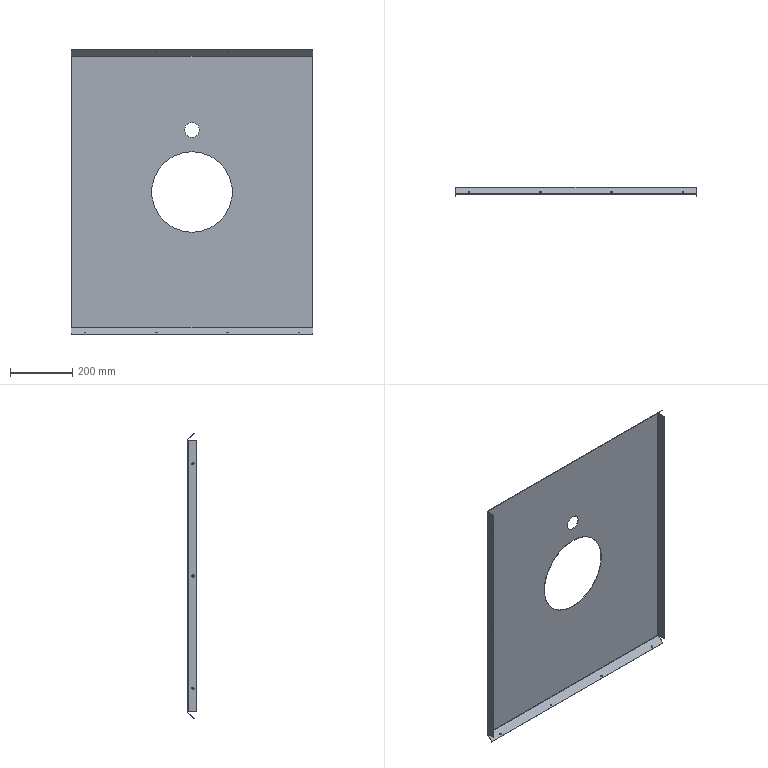Part | SolidWorks | features HoleWzd 3, EdgeFlange 2, Cut 1, FlatPattern 1, ICE 1, SMBaseFlange 1, SheetMetal 1 | 1 solid | 74 faces | box 780 x 30 x 921.426 mm | volume 870668 mm3 | cylinder 40 | plane 34 | commonest cylinder face diameters 5 x16 7 x12 2 x4 4.4 x4 48 x2 260 x2